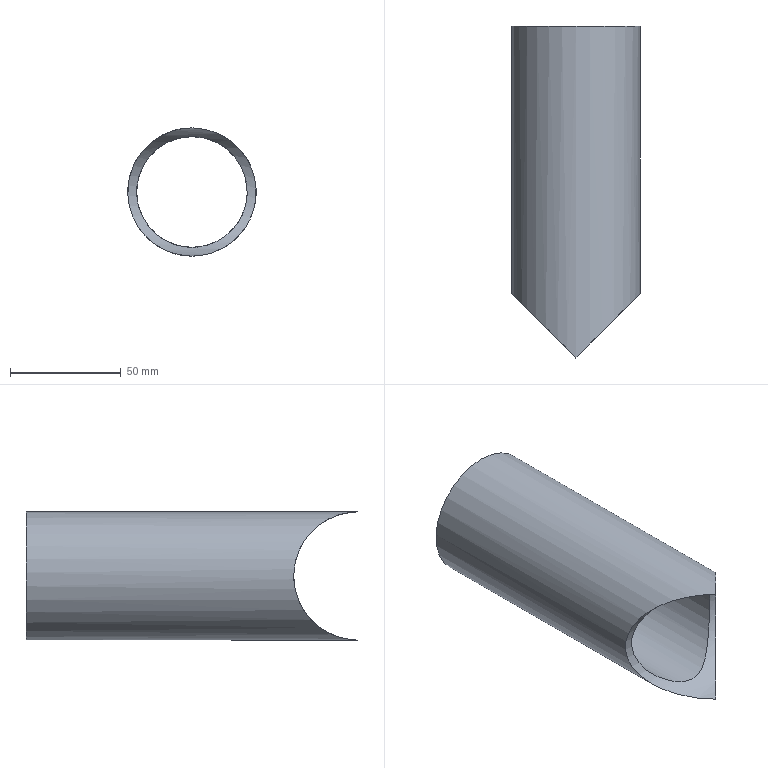Part | STEP file | JBJ-P-1004-02 | 1 solid | 5 faces | box 58 x 150 x 58 mm | volume 86410 mm3 | cylinder 4 | cone 1 | commonest cylinder face diameters 58 x2 3.3 x1 50 x1
STEP:
#1=CARTESIAN_POINT('',(29.,88.35,0.));
#2=VERTEX_POINT('',#1);
#3=CARTESIAN_POINT('',(29.,88.35,0.));
#4=CARTESIAN_POINT('',(29.,88.35,0.109));
#5=CARTESIAN_POINT('',(28.999,88.361,0.2162));
#6=CARTESIAN_POINT('',(28.997,88.403,0.4271));
#7=CARTESIAN_POINT('',(28.995,88.434,0.5319));
#8=CARTESIAN_POINT('',(28.991,88.517,0.7317));
#9=CARTESIAN_POINT('',(28.988,88.568,0.8265));
#10=CARTESIAN_POINT('',(28.983,88.688,1.006));
#11=CARTESIAN_POINT('',(28.98,88.757,1.091));
#12=CARTESIAN_POINT('',(28.97,88.986,1.319));
#13=CARTESIAN_POINT('',(28.964,89.17,1.442));
#14=CARTESIAN_POINT('',(28.956,89.567,1.607));
#15=CARTESIAN_POINT('',(28.953,89.784,1.65));
#16=CARTESIAN_POINT('',(28.953,90.107,1.65));
#17=CARTESIAN_POINT('',(28.954,90.216,1.639));
#18=CARTESIAN_POINT('',(28.956,90.428,1.597));
#19=CARTESIAN_POINT('',(28.958,90.531,1.566));
#20=CARTESIAN_POINT('',(28.962,90.73,1.483));
#21=CARTESIAN_POINT('',(28.965,90.827,1.432));
#22=CARTESIAN_POINT('',(28.97,91.006,1.312));
#23=CARTESIAN_POINT('',(28.973,91.089,1.244));
#24=CARTESIAN_POINT('',(28.98,91.243,1.09));
#25=CARTESIAN_POINT('',(28.983,91.312,1.007));
#26=CARTESIAN_POINT('',(28.988,91.431,0.8282));
#27=CARTESIAN_POINT('',(28.991,91.483,0.7318));
#28=CARTESIAN_POINT('',(28.995,91.566,0.5319));
#29=CARTESIAN_POINT('',(28.997,91.597,0.4291));
#30=CARTESIAN_POINT('',(28.999,91.639,0.2176));
#31=CARTESIAN_POINT('',(29.,91.65,0.1083));
#32=CARTESIAN_POINT('',(29.,91.65,-0.2148));
#33=CARTESIAN_POINT('',(28.997,91.607,-0.4319));
#34=CARTESIAN_POINT('',(28.989,91.443,-0.8291));
#35=CARTESIAN_POINT('',(28.983,91.32,-1.013));
#36=CARTESIAN_POINT('',(28.974,91.092,-1.242));
#37=CARTESIAN_POINT('',(28.97,91.007,-1.311));
#38=CARTESIAN_POINT('',(28.965,90.828,-1.431));
#39=CARTESIAN_POINT('',(28.962,90.733,-1.482));
#40=CARTESIAN_POINT('',(28.958,90.533,-1.565));
#41=CARTESIAN_POINT('',(28.956,90.429,-1.597));
#42=CARTESIAN_POINT('',(28.954,90.218,-1.639));
#43=CARTESIAN_POINT('',(28.953,90.111,-1.65));
#44=CARTESIAN_POINT('',(28.953,89.784,-1.65));
#45=CARTESIAN_POINT('',(28.956,89.57,-1.608));
#46=CARTESIAN_POINT('',(28.962,89.27,-1.483));
#47=CARTESIAN_POINT('',(28.965,89.175,-1.433));
#48=CARTESIAN_POINT('',(28.97,88.995,-1.313));
#49=CARTESIAN_POINT('',(28.973,88.91,-1.244));
#50=CARTESIAN_POINT('',(28.983,88.682,-1.016));
#51=CARTESIAN_POINT('',(28.989,88.559,-0.8316));
#52=CARTESIAN_POINT('',(28.997,88.394,-0.4347));
#53=CARTESIAN_POINT('',(29.,88.35,-0.2181));
#54=CARTESIAN_POINT('',(29.,88.35,0.));
#55=B_SPLINE_CURVE_WITH_KNOTS('',3,(#3,#4,#5,#6,#7,#8,#9,#10,#11,#12,#13,#14,#15,#16,#17,#18,#19,#20,#21,#22,#23,#24,#25,#26,#27,#28,#29,#30,#31,#32,#33,#34,#35,#36,#37,#38,#39,#40,#41,#42,#43,#44,#45,#46,#47,#48,#49,#50,#51,#52,#53,#54),.UNSPECIFIED.,.T.,.F.,(4,2,2,2,2,2,2,2,2,2,2,2,2,2,2,2,2,2,2,2,2,2,2,2,2,4),(0.,0.0003224,0.0006449,0.0009673,0.00129,0.001935,0.00258,0.002902,0.003224,0.003547,0.003869,0.004192,0.004514,0.004837,0.005159,0.005804,0.006449,0.006771,0.007094,0.007416,0.007739,0.008384,0.008706,0.009028,0.009673,0.01032),.UNSPECIFIED.);
#56=EDGE_CURVE('',#2,#2,#55,.T.);
#57=ORIENTED_EDGE('',*,*,#56,.T.);
#58=EDGE_LOOP('',(#57));
#59=FACE_BOUND('',#58,.T.);
#60=CARTESIAN_POINT('',(0.,150.,29.));
#61=VERTEX_POINT('',#60);
#62=CARTESIAN_POINT('',(0.,150.,0.));
#63=DIRECTION('',(0.,1.,0.));
#64=DIRECTION('',(0.,0.,1.));
#65=AXIS2_PLACEMENT_3D('',#62,#63,#64);
#66=CIRCLE('',#65,29.);
#67=EDGE_CURVE('',#61,#61,#66,.T.);
#68=ORIENTED_EDGE('',*,*,#67,.F.);
#69=EDGE_LOOP('',(#68));
#70=FACE_OUTER_BOUND('',#69,.T.);
#71=CARTESIAN_POINT('',(0.,0.,-29.));
#72=VERTEX_POINT('',#71);
#73=CARTESIAN_POINT('',(0.,0.,29.));
#74=VERTEX_POINT('',#73);
#75=CARTESIAN_POINT('',(0.,0.,-29.));
#76=CARTESIAN_POINT('',(-58.,58.,-29.));
#77=CARTESIAN_POINT('',(-58.,58.,29.));
#78=CARTESIAN_POINT('',(0.,0.,29.));
#79=(BOUNDED_CURVE()B_SPLINE_CURVE(3,(#75,#76,#77,#78),.UNSPECIFIED.,.F.,.F.)B_SPLINE_CURVE_WITH_KNOTS((4,4),(1.571,4.712),.UNSPECIFIED.)CURVE()GEOMETRIC_REPRESENTATION_ITEM()RATIONAL_B_SPLINE_CURVE((1.,0.3333,0.3333,1.))REPRESENTATION_ITEM(''));
#80=EDGE_CURVE('',#72,#74,#79,.T.);
#81=ORIENTED_EDGE('',*,*,#80,.T.);
#82=CARTESIAN_POINT('',(0.,0.,29.));
#83=CARTESIAN_POINT('',(58.,58.,29.));
#84=CARTESIAN_POINT('',(58.,58.,-29.));
#85=CARTESIAN_POINT('',(0.,0.,-29.));
#86=(BOUNDED_CURVE()B_SPLINE_CURVE(3,(#82,#83,#84,#85),.UNSPECIFIED.,.F.,.F.)B_SPLINE_CURVE_WITH_KNOTS((4,4),(1.571,4.712),.UNSPECIFIED.)CURVE()GEOMETRIC_REPRESENTATION_ITEM()RATIONAL_B_SPLINE_CURVE((1.,0.3333,0.3333,1.))REPRESENTATION_ITEM(''));
#87=EDGE_CURVE('',#74,#72,#86,.T.);
#88=ORIENTED_EDGE('',*,*,#87,.T.);
#89=EDGE_LOOP('',(#81,#88));
#90=FACE_OUTER_BOUND('',#89,.T.);
#91=CARTESIAN_POINT('',(0.,150.,0.));
#92=DIRECTION('',(0.,-1.,0.));
#93=DIRECTION('',(0.,0.,-1.));
#94=AXIS2_PLACEMENT_3D('',#91,#92,#93);
#95=CYLINDRICAL_SURFACE('',#94,29.);
#96=ADVANCED_FACE('',(#59,#70,#90),#95,.T.);
#97=CARTESIAN_POINT('',(24.945,90.,1.65));
#98=VERTEX_POINT('',#97);
#99=CARTESIAN_POINT('',(24.945,90.,1.65));
#100=CARTESIAN_POINT('',(24.945,90.109,1.65));
#101=CARTESIAN_POINT('',(24.946,90.216,1.639));
#102=CARTESIAN_POINT('',(24.949,90.427,1.597));
#103=CARTESIAN_POINT('',(24.951,90.532,1.566));
#104=CARTESIAN_POINT('',(24.956,90.732,1.483));
#105=CARTESIAN_POINT('',(24.959,90.827,1.432));
#106=CARTESIAN_POINT('',(24.966,91.006,1.312));
#107=CARTESIAN_POINT('',(24.969,91.091,1.243));
#108=CARTESIAN_POINT('',(24.98,91.319,1.014));
#109=CARTESIAN_POINT('',(24.987,91.442,0.8304));
#110=CARTESIAN_POINT('',(24.997,91.607,0.4333));
#111=CARTESIAN_POINT('',(25.,91.65,0.2162));
#112=CARTESIAN_POINT('',(25.,91.65,-0.1068));
#113=CARTESIAN_POINT('',(24.999,91.639,-0.2161));
#114=CARTESIAN_POINT('',(24.997,91.597,-0.4277));
#115=CARTESIAN_POINT('',(24.995,91.566,-0.5306));
#116=CARTESIAN_POINT('',(24.99,91.483,-0.7304));
#117=CARTESIAN_POINT('',(24.986,91.432,-0.827));
#118=CARTESIAN_POINT('',(24.98,91.312,-1.006));
#119=CARTESIAN_POINT('',(24.976,91.244,-1.089));
#120=CARTESIAN_POINT('',(24.969,91.09,-1.243));
#121=CARTESIAN_POINT('',(24.966,91.007,-1.312));
#122=CARTESIAN_POINT('',(24.959,90.828,-1.431));
#123=CARTESIAN_POINT('',(24.956,90.732,-1.483));
#124=CARTESIAN_POINT('',(24.951,90.532,-1.566));
#125=CARTESIAN_POINT('',(24.949,90.429,-1.597));
#126=CARTESIAN_POINT('',(24.946,90.218,-1.639));
#127=CARTESIAN_POINT('',(24.945,90.108,-1.65));
#128=CARTESIAN_POINT('',(24.945,89.785,-1.65));
#129=CARTESIAN_POINT('',(24.948,89.568,-1.607));
#130=CARTESIAN_POINT('',(24.958,89.171,-1.443));
#131=CARTESIAN_POINT('',(24.966,88.987,-1.32));
#132=CARTESIAN_POINT('',(24.976,88.758,-1.092));
#133=CARTESIAN_POINT('',(24.98,88.689,-1.007));
#134=CARTESIAN_POINT('',(24.986,88.569,-0.8278));
#135=CARTESIAN_POINT('',(24.989,88.518,-0.733));
#136=CARTESIAN_POINT('',(24.995,88.435,-0.5335));
#137=CARTESIAN_POINT('',(24.997,88.403,-0.4286));
#138=CARTESIAN_POINT('',(24.999,88.361,-0.2177));
#139=CARTESIAN_POINT('',(25.,88.35,-0.1105));
#140=CARTESIAN_POINT('',(25.,88.35,0.2161));
#141=CARTESIAN_POINT('',(24.997,88.392,0.4304));
#142=CARTESIAN_POINT('',(24.99,88.517,0.7305));
#143=CARTESIAN_POINT('',(24.987,88.567,0.8253));
#144=CARTESIAN_POINT('',(24.98,88.687,1.005));
#145=CARTESIAN_POINT('',(24.976,88.756,1.09));
#146=CARTESIAN_POINT('',(24.966,88.984,1.318));
#147=CARTESIAN_POINT('',(24.959,89.168,1.441));
#148=CARTESIAN_POINT('',(24.948,89.565,1.606));
#149=CARTESIAN_POINT('',(24.945,89.782,1.65));
#150=CARTESIAN_POINT('',(24.945,90.,1.65));
#151=B_SPLINE_CURVE_WITH_KNOTS('',3,(#99,#100,#101,#102,#103,#104,#105,#106,#107,#108,#109,#110,#111,#112,#113,#114,#115,#116,#117,#118,#119,#120,#121,#122,#123,#124,#125,#126,#127,#128,#129,#130,#131,#132,#133,#134,#135,#136,#137,#138,#139,#140,#141,#142,#143,#144,#145,#146,#147,#148,#149,#150),.UNSPECIFIED.,.T.,.F.,(4,2,2,2,2,2,2,2,2,2,2,2,2,2,2,2,2,2,2,2,2,2,2,2,2,4),(0.,0.0003225,0.0006449,0.0009674,0.00129,0.001935,0.00258,0.002902,0.003225,0.003547,0.00387,0.004192,0.004515,0.004837,0.005159,0.005804,0.006449,0.006772,0.007094,0.007417,0.007739,0.008384,0.008707,0.009029,0.009674,0.01032),.UNSPECIFIED.);
#152=EDGE_CURVE('',#98,#98,#151,.T.);
#153=ORIENTED_EDGE('',*,*,#152,.F.);
#154=EDGE_LOOP('',(#153));
#155=FACE_BOUND('',#154,.T.);
#156=CARTESIAN_POINT('',(0.,146.,25.));
#157=VERTEX_POINT('',#156);
#158=CARTESIAN_POINT('',(0.,146.,0.));
#159=DIRECTION('',(0.,1.,0.));
#160=DIRECTION('',(0.,0.,1.));
#161=AXIS2_PLACEMENT_3D('',#158,#159,#160);
#162=CIRCLE('',#161,25.);
#163=EDGE_CURVE('',#157,#157,#162,.T.);
#164=ORIENTED_EDGE('',*,*,#163,.T.);
#165=EDGE_LOOP('',(#164));
#166=FACE_OUTER_BOUND('',#165,.T.);
#167=CARTESIAN_POINT('',(0.,14.697,-25.));
#168=VERTEX_POINT('',#167);
#169=CARTESIAN_POINT('',(0.,14.697,-25.));
#170=CARTESIAN_POINT('',(-0.894,14.697,-25.));
#171=CARTESIAN_POINT('',(-1.77,14.779,-24.952));
#172=CARTESIAN_POINT('',(-3.061,15.006,-24.816));
#173=CARTESIAN_POINT('',(-3.487,15.1,-24.759));
#174=CARTESIAN_POINT('',(-4.333,15.317,-24.625));
#175=CARTESIAN_POINT('',(-4.754,15.442,-24.547));
#176=CARTESIAN_POINT('',(-5.995,15.853,-24.285));
#177=CARTESIAN_POINT('',(-6.787,16.174,-24.074));
#178=CARTESIAN_POINT('',(-8.323,16.876,-23.588));
#179=CARTESIAN_POINT('',(-9.065,17.257,-23.312));
#180=CARTESIAN_POINT('',(-10.511,18.059,-22.697));
#181=CARTESIAN_POINT('',(-11.216,18.48,-22.356));
#182=CARTESIAN_POINT('',(-12.574,19.335,-21.622));
#183=CARTESIAN_POINT('',(-13.228,19.768,-21.227));
#184=CARTESIAN_POINT('',(-15.126,21.07,-19.963));
#185=CARTESIAN_POINT('',(-16.308,21.942,-19.012));
#186=CARTESIAN_POINT('',(-17.691,22.998,-17.669));
#187=CARTESIAN_POINT('',(-17.962,23.208,-17.393));
#188=CARTESIAN_POINT('',(-18.496,23.624,-16.824));
#189=CARTESIAN_POINT('',(-18.759,23.83,-16.53));
#190=CARTESIAN_POINT('',(-19.525,24.436,-15.633));
#191=CARTESIAN_POINT('',(-20.009,24.825,-15.009));
#192=CARTESIAN_POINT('',(-21.379,25.938,-13.056));
#193=CARTESIAN_POINT('',(-22.185,26.609,-11.647));
#194=CARTESIAN_POINT('',(-23.546,27.754,-8.567));
#195=CARTESIAN_POINT('',(-24.076,28.207,-6.954));
#196=CARTESIAN_POINT('',(-24.532,28.597,-4.834));
#197=CARTESIAN_POINT('',(-24.613,28.667,-4.405));
#198=CARTESIAN_POINT('',(-24.753,28.787,-3.536));
#199=CARTESIAN_POINT('',(-24.811,28.837,-3.097));
#200=CARTESIAN_POINT('',(-24.952,28.958,-1.785));
#201=CARTESIAN_POINT('',(-24.999,28.999,-0.9102));
#202=CARTESIAN_POINT('',(-25.001,29.001,0.8417));
#203=CARTESIAN_POINT('',(-24.956,28.962,1.718));
#204=CARTESIAN_POINT('',(-24.819,28.844,3.035));
#205=CARTESIAN_POINT('',(-24.761,28.794,3.475));
#206=CARTESIAN_POINT('',(-24.624,28.676,4.342));
#207=CARTESIAN_POINT('',(-24.544,28.608,4.771));
#208=CARTESIAN_POINT('',(-24.274,28.376,6.044));
#209=CARTESIAN_POINT('',(-24.052,28.186,6.873));
#210=CARTESIAN_POINT('',(-23.658,27.852,8.091));
#211=CARTESIAN_POINT('',(-23.517,27.732,8.492));
#212=CARTESIAN_POINT('',(-23.215,27.476,9.286));
#213=CARTESIAN_POINT('',(-23.054,27.34,9.679));
#214=CARTESIAN_POINT('',(-22.21,26.63,11.598));
#215=CARTESIAN_POINT('',(-21.406,25.96,13.014));
#216=CARTESIAN_POINT('',(-20.255,25.025,14.659));
#217=CARTESIAN_POINT('',(-20.017,24.833,14.982));
#218=CARTESIAN_POINT('',(-19.531,24.443,15.611));
#219=CARTESIAN_POINT('',(-19.283,24.244,15.917));
#220=CARTESIAN_POINT('',(-18.521,23.641,16.811));
#221=CARTESIAN_POINT('',(-17.991,23.229,17.375));
#222=CARTESIAN_POINT('',(-16.341,21.966,18.982));
#223=CARTESIAN_POINT('',(-15.158,21.093,19.94));
#224=CARTESIAN_POINT('',(-13.242,19.777,21.219));
#225=CARTESIAN_POINT('',(-12.581,19.339,21.618));
#226=CARTESIAN_POINT('',(-11.225,18.486,22.352));
#227=CARTESIAN_POINT('',(-10.528,18.069,22.688));
#228=CARTESIAN_POINT('',(-9.09,17.27,23.302));
#229=CARTESIAN_POINT('',(-8.347,16.888,23.579));
#230=CARTESIAN_POINT('',(-6.803,16.181,24.07));
#231=CARTESIAN_POINT('',(-5.998,15.855,24.284));
#232=CARTESIAN_POINT('',(-4.355,15.309,24.632));
#233=CARTESIAN_POINT('',(-3.512,15.087,24.767));
#234=CARTESIAN_POINT('',(-2.209,14.856,24.906));
#235=CARTESIAN_POINT('',(-1.766,14.796,24.941));
#236=CARTESIAN_POINT('',(-0.8843,14.717,24.988));
#237=CARTESIAN_POINT('',(-0.4445,14.697,25.));
#238=CARTESIAN_POINT('',(0.8722,14.697,25.));
#239=CARTESIAN_POINT('',(1.746,14.775,24.954));
#240=CARTESIAN_POINT('',(3.053,15.005,24.817));
#241=CARTESIAN_POINT('',(3.486,15.099,24.759));
#242=CARTESIAN_POINT('',(4.333,15.317,24.625));
#243=CARTESIAN_POINT('',(4.749,15.44,24.548));
#244=CARTESIAN_POINT('',(5.977,15.847,24.289));
#245=CARTESIAN_POINT('',(6.77,16.167,24.08));
#246=CARTESIAN_POINT('',(7.93,16.696,23.712));
#247=CARTESIAN_POINT('',(8.313,16.882,23.581));
#248=CARTESIAN_POINT('',(9.062,17.263,23.303));
#249=CARTESIAN_POINT('',(9.43,17.459,23.157));
#250=CARTESIAN_POINT('',(11.234,18.46,22.389));
#251=CARTESIAN_POINT('',(12.575,19.321,21.661));
#252=CARTESIAN_POINT('',(14.481,20.627,20.393));
#253=CARTESIAN_POINT('',(15.098,21.066,19.941));
#254=CARTESIAN_POINT('',(16.297,21.942,18.974));
#255=CARTESIAN_POINT('',(16.872,22.373,18.464));
#256=CARTESIAN_POINT('',(18.527,23.638,16.856));
#257=CARTESIAN_POINT('',(19.538,24.442,15.678));
#258=CARTESIAN_POINT('',(20.909,25.556,13.728));
#259=CARTESIAN_POINT('',(21.343,25.912,13.045));
#260=CARTESIAN_POINT('',(22.154,26.584,11.615));
#261=CARTESIAN_POINT('',(22.525,26.895,10.877));
#262=CARTESIAN_POINT('',(23.198,27.461,9.356));
#263=CARTESIAN_POINT('',(23.5,27.717,8.572));
#264=CARTESIAN_POINT('',(23.897,28.054,7.357));
#265=CARTESIAN_POINT('',(24.019,28.159,6.946));
#266=CARTESIAN_POINT('',(24.246,28.352,6.111));
#267=CARTESIAN_POINT('',(24.349,28.441,5.685));
#268=CARTESIAN_POINT('',(24.807,28.833,3.557));
#269=CARTESIAN_POINT('',(24.996,28.996,1.825));
#270=CARTESIAN_POINT('',(25.002,29.002,-0.82));
#271=CARTESIAN_POINT('',(24.957,28.963,-1.715));
#272=CARTESIAN_POINT('',(24.774,28.806,-3.465));
#273=CARTESIAN_POINT('',(24.638,28.689,-4.325));
#274=CARTESIAN_POINT('',(24.28,28.381,-6.02));
#275=CARTESIAN_POINT('',(24.057,28.191,-6.855));
#276=CARTESIAN_POINT('',(23.529,27.741,-8.494));
#277=CARTESIAN_POINT('',(23.227,27.486,-9.285));
#278=CARTESIAN_POINT('',(22.556,26.921,-10.813));
#279=CARTESIAN_POINT('',(22.187,26.612,-11.551));
#280=CARTESIAN_POINT('',(21.383,25.946,-12.979));
#281=CARTESIAN_POINT('',(20.947,25.587,-13.67));
#282=CARTESIAN_POINT('',(19.571,24.47,-15.637));
#283=CARTESIAN_POINT('',(18.56,23.663,-16.82));
#284=CARTESIAN_POINT('',(16.906,22.399,-18.433));
#285=CARTESIAN_POINT('',(16.332,21.968,-18.943));
#286=CARTESIAN_POINT('',(15.136,21.093,-19.912));
#287=CARTESIAN_POINT('',(14.516,20.652,-20.368));
#288=CARTESIAN_POINT('',(12.609,19.342,-21.641));
#289=CARTESIAN_POINT('',(11.268,18.481,-22.372));
#290=CARTESIAN_POINT('',(9.109,17.28,-23.295));
#291=CARTESIAN_POINT('',(8.364,16.896,-23.574));
#292=CARTESIAN_POINT('',(6.809,16.183,-24.069));
#293=CARTESIAN_POINT('',(6.013,15.861,-24.28));
#294=CARTESIAN_POINT('',(4.373,15.314,-24.629));
#295=CARTESIAN_POINT('',(3.528,15.09,-24.765));
#296=CARTESIAN_POINT('',(1.778,14.779,-24.952));
#297=CARTESIAN_POINT('',(0.894,14.697,-25.));
#298=CARTESIAN_POINT('',(0.,14.697,-25.));
#299=B_SPLINE_CURVE_WITH_KNOTS('',3,(#169,#170,#171,#172,#173,#174,#175,#176,#177,#178,#179,#180,#181,#182,#183,#184,#185,#186,#187,#188,#189,#190,#191,#192,#193,#194,#195,#196,#197,#198,#199,#200,#201,#202,#203,#204,#205,#206,#207,#208,#209,#210,#211,#212,#213,#214,#215,#216,#217,#218,#219,#220,#221,#222,#223,#224,#225,#226,#227,#228,#229,#230,#231,#232,#233,#234,#235,#236,#237,#238,#239,#240,#241,#242,#243,#244,#245,#246,#247,#248,#249,#250,#251,#252,#253,#254,#255,#256,#257,#258,#259,#260,#261,#262,#263,#264,#265,#266,#267,#268,#269,#270,#271,#272,#273,#274,#275,#276,#277,#278,#279,#280,#281,#282,#283,#284,#285,#286,#287,#288,#289,#290,#291,#292,#293,#294,#295,#296,#297,#298),.UNSPECIFIED.,.T.,.F.,(4,2,2,2,2,2,2,2,2,2,2,2,2,2,2,2,2,2,2,2,2,2,2,2,2,2,2,2,2,2,2,2,2,2,2,2,2,2,2,2,2,2,2,2,2,2,2,2,2,2,2,2,2,2,2,2,2,2,2,2,2,2,2,2,4),(0.,0.002635,0.003953,0.005271,0.007906,0.01054,0.01318,0.01581,0.02108,0.0224,0.02372,0.02635,0.03162,0.0369,0.03821,0.03953,0.04217,0.0448,0.04612,0.04744,0.05007,0.05139,0.05271,0.05798,0.0593,0.06061,0.06325,0.06852,0.07115,0.07379,0.07643,0.07906,0.0817,0.08301,0.08433,0.08697,0.08828,0.0896,0.09224,0.09356,0.09487,0.1001,0.1028,0.1054,0.1107,0.1133,0.116,0.1186,0.1199,0.1212,0.1265,0.1291,0.1318,0.1344,0.137,0.1397,0.1423,0.1476,0.1502,0.1529,0.1581,0.1608,0.1634,0.166,0.1687),.UNSPECIFIED.);
#300=EDGE_CURVE('',#168,#168,#299,.T.);
#301=ORIENTED_EDGE('',*,*,#300,.F.);
#302=EDGE_LOOP('',(#301));
#303=FACE_OUTER_BOUND('',#302,.T.);
#304=CARTESIAN_POINT('',(0.,150.,0.));
#305=DIRECTION('',(0.,-1.,0.));
#306=DIRECTION('',(0.,0.,-1.));
#307=AXIS2_PLACEMENT_3D('',#304,#305,#306);
#308=CYLINDRICAL_SURFACE('',#307,25.);
#309=ADVANCED_FACE('',(#155,#166,#303),#308,.F.);
#310=ORIENTED_EDGE('',*,*,#300,.T.);
#311=EDGE_LOOP('',(#310));
#312=FACE_BOUND('',#311,.T.);
#313=ORIENTED_EDGE('',*,*,#80,.F.);
#314=ORIENTED_EDGE('',*,*,#87,.F.);
#315=EDGE_LOOP('',(#313,#314));
#316=FACE_OUTER_BOUND('',#315,.T.);
#317=CARTESIAN_POINT('',(-29.,0.,0.));
#318=DIRECTION('',(1.,0.,0.));
#319=DIRECTION('',(0.,0.,-1.));
#320=AXIS2_PLACEMENT_3D('',#317,#318,#319);
#321=CYLINDRICAL_SURFACE('',#320,29.);
#322=ADVANCED_FACE('',(#312,#316),#321,.F.);
#323=ORIENTED_EDGE('',*,*,#67,.T.);
#324=EDGE_LOOP('',(#323));
#325=FACE_OUTER_BOUND('',#324,.T.);
#326=ORIENTED_EDGE('',*,*,#163,.F.);
#327=EDGE_LOOP('',(#326));
#328=FACE_BOUND('',#327,.T.);
#329=CARTESIAN_POINT('',(0.,146.,0.));
#330=DIRECTION('',(0.,1.,0.));
#331=DIRECTION('',(0.,0.,1.));
#332=AXIS2_PLACEMENT_3D('',#329,#330,#331);
#333=CONICAL_SURFACE('',#332,25.,0.7854);
#334=ADVANCED_FACE('',(#325,#328),#333,.F.);
#335=ORIENTED_EDGE('',*,*,#152,.T.);
#336=EDGE_LOOP('',(#335));
#337=FACE_OUTER_BOUND('',#336,.T.);
#338=ORIENTED_EDGE('',*,*,#56,.F.);
#339=EDGE_LOOP('',(#338));
#340=FACE_OUTER_BOUND('',#339,.T.);
#341=CARTESIAN_POINT('',(0.,90.,0.));
#342=DIRECTION('',(-1.,0.,0.));
#343=DIRECTION('',(0.,0.,1.));
#344=AXIS2_PLACEMENT_3D('',#341,#342,#343);
#345=CYLINDRICAL_SURFACE('',#344,1.65);
#346=ADVANCED_FACE('',(#337,#340),#345,.F.);
#347=CLOSED_SHELL('',(#96,#309,#322,#334,#346));
#348=MANIFOLD_SOLID_BREP('',#347);
#349=CARTESIAN_POINT('',(0.,0.,0.));
#350=DIRECTION('',(0.,0.,1.));
#351=DIRECTION('',(1.,0.,0.));
#352=AXIS2_PLACEMENT_3D('',#349,#350,#351);
#353=(LENGTH_UNIT()NAMED_UNIT(*)SI_UNIT(.MILLI.,.METRE.));
#354=UNCERTAINTY_MEASURE_WITH_UNIT(LENGTH_MEASURE(0.00001),#353,'','');
#355=(NAMED_UNIT(*)PLANE_ANGLE_UNIT()SI_UNIT($,.RADIAN.));
#356=(NAMED_UNIT(*)SI_UNIT($,.STERADIAN.)SOLID_ANGLE_UNIT());
#357=(GEOMETRIC_REPRESENTATION_CONTEXT(3)GLOBAL_UNCERTAINTY_ASSIGNED_CONTEXT((#354))GLOBAL_UNIT_ASSIGNED_CONTEXT((#353,#355,#356))REPRESENTATION_CONTEXT('',''));
#358=ADVANCED_BREP_SHAPE_REPRESENTATION('',(#348,#352),#357);